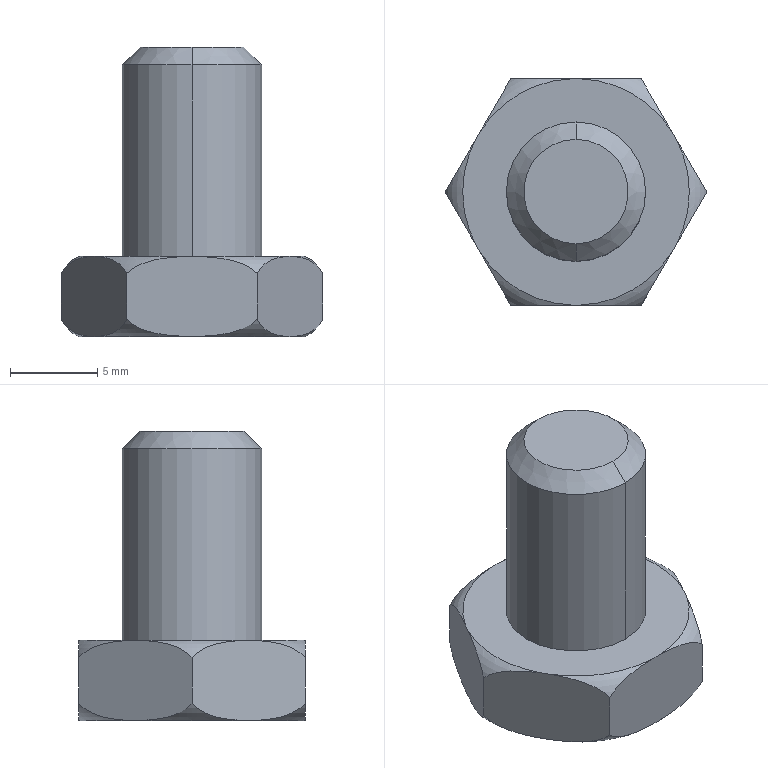Part | NX | features solid 2 | 1 solid | 25 faces | box 15.011 x 13 x 16.6 mm | volume 1260 mm3 | torus 12 | plane 9 | cylinder 2 | cone 2 | commonest cylinder face diameters 8 x2
STEP:
#1=CARTESIAN_POINT('',(280.505,2120.638,-1073.6));
#2=VERTEX_POINT('',#1);
#3=CARTESIAN_POINT('',(280.236,2120.172,-1073.6));
#4=VERTEX_POINT('',#3);
#5=CARTESIAN_POINT('',(280.505,2120.638,-1073.6));
#6=DIRECTION('',(-0.5,-0.866,0.));
#7=VECTOR('',#6,1000.);
#8=LINE('',#5,#7);
#9=EDGE_CURVE('',#2,#4,#8,.T.);
#10=ORIENTED_EDGE('',*,*,#9,.F.);
#11=CARTESIAN_POINT('',(285.731,2123.655,-1073.6));
#12=VERTEX_POINT('',#11);
#13=CARTESIAN_POINT('',(286.,2117.155,-1073.6));
#14=DIRECTION('',(0.,0.,1.));
#15=DIRECTION('',(-0.04131,0.9991,0.));
#16=AXIS2_PLACEMENT_3D('',#13,#14,#15);
#17=CIRCLE('',#16,6.506);
#18=EDGE_CURVE('',#12,#2,#17,.T.);
#19=ORIENTED_EDGE('',*,*,#18,.F.);
#20=CARTESIAN_POINT('',(286.269,2123.655,-1073.6));
#21=VERTEX_POINT('',#20);
#22=CARTESIAN_POINT('',(286.269,2123.655,-1073.6));
#23=DIRECTION('',(-1.,0.,0.));
#24=VECTOR('',#23,1000.);
#25=LINE('',#22,#24);
#26=EDGE_CURVE('',#21,#12,#25,.T.);
#27=ORIENTED_EDGE('',*,*,#26,.F.);
#28=CARTESIAN_POINT('',(291.495,2120.638,-1073.6));
#29=VERTEX_POINT('',#28);
#30=CARTESIAN_POINT('',(286.,2117.155,-1073.6));
#31=DIRECTION('',(0.,0.,1.));
#32=DIRECTION('',(0.8446,0.5353,0.));
#33=AXIS2_PLACEMENT_3D('',#30,#31,#32);
#34=CIRCLE('',#33,6.506);
#35=EDGE_CURVE('',#29,#21,#34,.T.);
#36=ORIENTED_EDGE('',*,*,#35,.F.);
#37=CARTESIAN_POINT('',(291.764,2120.172,-1073.6));
#38=VERTEX_POINT('',#37);
#39=CARTESIAN_POINT('',(291.764,2120.172,-1073.6));
#40=DIRECTION('',(-0.5,0.866,0.));
#41=VECTOR('',#40,1000.);
#42=LINE('',#39,#41);
#43=EDGE_CURVE('',#38,#29,#42,.T.);
#44=ORIENTED_EDGE('',*,*,#43,.F.);
#45=CARTESIAN_POINT('',(292.506,2117.155,-1073.6));
#46=VERTEX_POINT('',#45);
#47=CARTESIAN_POINT('',(286.,2117.155,-1073.6));
#48=DIRECTION('',(0.,0.,1.));
#49=DIRECTION('',(1.,0.,0.));
#50=AXIS2_PLACEMENT_3D('',#47,#48,#49);
#51=CIRCLE('',#50,6.506);
#52=EDGE_CURVE('',#46,#38,#51,.T.);
#53=ORIENTED_EDGE('',*,*,#52,.F.);
#54=CARTESIAN_POINT('',(291.764,2114.138,-1073.6));
#55=VERTEX_POINT('',#54);
#56=CARTESIAN_POINT('',(286.,2117.155,-1073.6));
#57=DIRECTION('',(0.,0.,1.));
#58=DIRECTION('',(0.8859,-0.4638,0.));
#59=AXIS2_PLACEMENT_3D('',#56,#57,#58);
#60=CIRCLE('',#59,6.506);
#61=EDGE_CURVE('',#55,#46,#60,.T.);
#62=ORIENTED_EDGE('',*,*,#61,.F.);
#63=CARTESIAN_POINT('',(291.495,2113.672,-1073.6));
#64=VERTEX_POINT('',#63);
#65=CARTESIAN_POINT('',(291.495,2113.672,-1073.6));
#66=DIRECTION('',(0.5,0.866,0.));
#67=VECTOR('',#66,1000.);
#68=LINE('',#65,#67);
#69=EDGE_CURVE('',#64,#55,#68,.T.);
#70=ORIENTED_EDGE('',*,*,#69,.F.);
#71=CARTESIAN_POINT('',(286.269,2110.655,-1073.6));
#72=VERTEX_POINT('',#71);
#73=CARTESIAN_POINT('',(286.,2117.155,-1073.6));
#74=DIRECTION('',(0.,0.,1.));
#75=DIRECTION('',(0.04131,-0.9991,0.));
#76=AXIS2_PLACEMENT_3D('',#73,#74,#75);
#77=CIRCLE('',#76,6.506);
#78=EDGE_CURVE('',#72,#64,#77,.T.);
#79=ORIENTED_EDGE('',*,*,#78,.F.);
#80=CARTESIAN_POINT('',(285.731,2110.655,-1073.6));
#81=VERTEX_POINT('',#80);
#82=CARTESIAN_POINT('',(285.731,2110.655,-1073.6));
#83=DIRECTION('',(1.,0.,0.));
#84=VECTOR('',#83,1000.);
#85=LINE('',#82,#84);
#86=EDGE_CURVE('',#81,#72,#85,.T.);
#87=ORIENTED_EDGE('',*,*,#86,.F.);
#88=CARTESIAN_POINT('',(280.505,2113.672,-1073.6));
#89=VERTEX_POINT('',#88);
#90=CARTESIAN_POINT('',(286.,2117.155,-1073.6));
#91=DIRECTION('',(0.,0.,1.));
#92=DIRECTION('',(-0.8446,-0.5353,0.));
#93=AXIS2_PLACEMENT_3D('',#90,#91,#92);
#94=CIRCLE('',#93,6.506);
#95=EDGE_CURVE('',#89,#81,#94,.T.);
#96=ORIENTED_EDGE('',*,*,#95,.F.);
#97=CARTESIAN_POINT('',(280.236,2114.138,-1073.6));
#98=VERTEX_POINT('',#97);
#99=CARTESIAN_POINT('',(280.236,2114.138,-1073.6));
#100=DIRECTION('',(0.5,-0.866,0.));
#101=VECTOR('',#100,1000.);
#102=LINE('',#99,#101);
#103=EDGE_CURVE('',#98,#89,#102,.T.);
#104=ORIENTED_EDGE('',*,*,#103,.F.);
#105=CARTESIAN_POINT('',(279.494,2117.155,-1073.6));
#106=VERTEX_POINT('',#105);
#107=CARTESIAN_POINT('',(286.,2117.155,-1073.6));
#108=DIRECTION('',(0.,0.,1.));
#109=DIRECTION('',(-1.,0.,0.));
#110=AXIS2_PLACEMENT_3D('',#107,#108,#109);
#111=CIRCLE('',#110,6.506);
#112=EDGE_CURVE('',#106,#98,#111,.T.);
#113=ORIENTED_EDGE('',*,*,#112,.F.);
#114=CARTESIAN_POINT('',(286.,2117.155,-1073.6));
#115=DIRECTION('',(0.,0.,1.));
#116=DIRECTION('',(-0.8859,0.4638,0.));
#117=AXIS2_PLACEMENT_3D('',#114,#115,#116);
#118=CIRCLE('',#117,6.506);
#119=EDGE_CURVE('',#4,#106,#118,.T.);
#120=ORIENTED_EDGE('',*,*,#119,.F.);
#121=EDGE_LOOP('',(#10,#19,#27,#36,#44,#53,#62,#70,#79,#87,#96,#104,#113,#120));
#122=FACE_BOUND('',#121,.T.);
#123=CARTESIAN_POINT('',(286.,2117.155,-1073.6));
#124=DIRECTION('',(0.,0.,1.));
#125=DIRECTION('',(1.,0.,0.));
#126=AXIS2_PLACEMENT_3D('',#123,#124,#125);
#127=PLANE('',#126);
#128=ADVANCED_FACE('',(#122),#127,.F.);
#129=CARTESIAN_POINT('',(278.494,2117.155,-1072.6));
#130=VERTEX_POINT('',#129);
#131=CARTESIAN_POINT('',(278.494,2117.155,-1072.6));
#132=CARTESIAN_POINT('',(278.513,2117.123,-1072.641));
#133=CARTESIAN_POINT('',(278.553,2117.053,-1072.722));
#134=CARTESIAN_POINT('',(278.626,2116.927,-1072.843));
#135=CARTESIAN_POINT('',(278.713,2116.776,-1072.962));
#136=CARTESIAN_POINT('',(278.817,2116.596,-1073.079));
#137=CARTESIAN_POINT('',(278.94,2116.383,-1073.191));
#138=CARTESIAN_POINT('',(279.081,2116.139,-1073.292));
#139=CARTESIAN_POINT('',(279.239,2115.866,-1073.381));
#140=CARTESIAN_POINT('',(279.413,2115.565,-1073.455));
#141=CARTESIAN_POINT('',(279.602,2115.236,-1073.514));
#142=CARTESIAN_POINT('',(279.805,2114.886,-1073.558));
#143=CARTESIAN_POINT('',(280.017,2114.517,-1073.587));
#144=CARTESIAN_POINT('',(280.163,2114.266,-1073.597));
#145=CARTESIAN_POINT('',(280.236,2114.138,-1073.6));
#146=B_SPLINE_CURVE_WITH_KNOTS('',3,(#131,#132,#133,#134,#135,#136,#137,#138,#139,#140,#141,#142,#143,#144,#145),.UNSPECIFIED.,.F.,.F.,(4,1,1,1,1,1,1,1,1,1,1,1,4),(0.,0.08333,0.1667,0.25,0.3333,0.4167,0.5,0.5833,0.6667,0.75,0.8333,0.9167,1.),.QUASI_UNIFORM_KNOTS.);
#147=EDGE_CURVE('',#130,#98,#146,.T.);
#148=ORIENTED_EDGE('',*,*,#147,.F.);
#149=CARTESIAN_POINT('',(278.494,2117.155,-1072.6));
#150=CARTESIAN_POINT('',(278.513,2117.187,-1072.641));
#151=CARTESIAN_POINT('',(278.553,2117.257,-1072.722));
#152=CARTESIAN_POINT('',(278.626,2117.383,-1072.843));
#153=CARTESIAN_POINT('',(278.713,2117.534,-1072.962));
#154=CARTESIAN_POINT('',(278.817,2117.715,-1073.079));
#155=CARTESIAN_POINT('',(278.94,2117.927,-1073.191));
#156=CARTESIAN_POINT('',(279.081,2118.171,-1073.292));
#157=CARTESIAN_POINT('',(279.239,2118.444,-1073.381));
#158=CARTESIAN_POINT('',(279.413,2118.745,-1073.455));
#159=CARTESIAN_POINT('',(279.602,2119.074,-1073.514));
#160=CARTESIAN_POINT('',(279.805,2119.424,-1073.558));
#161=CARTESIAN_POINT('',(280.017,2119.793,-1073.587));
#162=CARTESIAN_POINT('',(280.163,2120.044,-1073.597));
#163=CARTESIAN_POINT('',(280.236,2120.172,-1073.6));
#164=B_SPLINE_CURVE_WITH_KNOTS('',3,(#149,#150,#151,#152,#153,#154,#155,#156,#157,#158,#159,#160,#161,#162,#163),.UNSPECIFIED.,.F.,.F.,(4,1,1,1,1,1,1,1,1,1,1,1,4),(0.,0.08333,0.1667,0.25,0.3333,0.4167,0.5,0.5833,0.6667,0.75,0.8333,0.9167,1.),.QUASI_UNIFORM_KNOTS.);
#165=EDGE_CURVE('',#130,#4,#164,.T.);
#166=ORIENTED_EDGE('',*,*,#165,.T.);
#167=ORIENTED_EDGE('',*,*,#119,.T.);
#168=ORIENTED_EDGE('',*,*,#112,.T.);
#169=EDGE_LOOP('',(#148,#166,#167,#168));
#170=FACE_BOUND('',#169,.T.);
#171=CARTESIAN_POINT('',(286.,2117.155,-1071.777));
#172=DIRECTION('',(0.,0.,1.));
#173=DIRECTION('',(1.,0.,0.));
#174=AXIS2_PLACEMENT_3D('',#171,#172,#173);
#175=TOROIDAL_SURFACE('',#174,5.683,2.);
#176=ADVANCED_FACE('',(#170),#175,.T.);
#177=CARTESIAN_POINT('',(280.236,2120.172,-1069.));
#178=VERTEX_POINT('',#177);
#179=CARTESIAN_POINT('',(280.505,2120.638,-1069.));
#180=VERTEX_POINT('',#179);
#181=CARTESIAN_POINT('',(280.236,2120.172,-1069.));
#182=DIRECTION('',(0.5,0.866,0.));
#183=VECTOR('',#182,1000.);
#184=LINE('',#181,#183);
#185=EDGE_CURVE('',#178,#180,#184,.T.);
#186=ORIENTED_EDGE('',*,*,#185,.T.);
#187=CARTESIAN_POINT('',(282.247,2123.655,-1070.));
#188=VERTEX_POINT('',#187);
#189=CARTESIAN_POINT('',(282.247,2123.655,-1070.));
#190=CARTESIAN_POINT('',(282.229,2123.623,-1069.959));
#191=CARTESIAN_POINT('',(282.188,2123.553,-1069.878));
#192=CARTESIAN_POINT('',(282.116,2123.427,-1069.757));
#193=CARTESIAN_POINT('',(282.028,2123.276,-1069.638));
#194=CARTESIAN_POINT('',(281.924,2123.095,-1069.521));
#195=CARTESIAN_POINT('',(281.801,2122.883,-1069.409));
#196=CARTESIAN_POINT('',(281.66,2122.639,-1069.308));
#197=CARTESIAN_POINT('',(281.503,2122.366,-1069.219));
#198=CARTESIAN_POINT('',(281.329,2122.065,-1069.145));
#199=CARTESIAN_POINT('',(281.139,2121.736,-1069.086));
#200=CARTESIAN_POINT('',(280.937,2121.386,-1069.042));
#201=CARTESIAN_POINT('',(280.724,2121.017,-1069.013));
#202=CARTESIAN_POINT('',(280.579,2120.766,-1069.003));
#203=CARTESIAN_POINT('',(280.505,2120.638,-1069.));
#204=B_SPLINE_CURVE_WITH_KNOTS('',3,(#189,#190,#191,#192,#193,#194,#195,#196,#197,#198,#199,#200,#201,#202,#203),.UNSPECIFIED.,.F.,.F.,(4,1,1,1,1,1,1,1,1,1,1,1,4),(0.,0.08333,0.1667,0.25,0.3333,0.4167,0.5,0.5833,0.6667,0.75,0.8333,0.9167,1.),.QUASI_UNIFORM_KNOTS.);
#205=EDGE_CURVE('',#188,#180,#204,.T.);
#206=ORIENTED_EDGE('',*,*,#205,.F.);
#207=CARTESIAN_POINT('',(282.247,2123.655,-1072.6));
#208=VERTEX_POINT('',#207);
#209=CARTESIAN_POINT('',(282.247,2123.655,-1072.6));
#210=DIRECTION('',(0.,0.,1.));
#211=VECTOR('',#210,1000.);
#212=LINE('',#209,#211);
#213=EDGE_CURVE('',#208,#188,#212,.T.);
#214=ORIENTED_EDGE('',*,*,#213,.F.);
#215=CARTESIAN_POINT('',(282.247,2123.655,-1072.6));
#216=CARTESIAN_POINT('',(282.229,2123.623,-1072.641));
#217=CARTESIAN_POINT('',(282.188,2123.553,-1072.722));
#218=CARTESIAN_POINT('',(282.116,2123.427,-1072.843));
#219=CARTESIAN_POINT('',(282.028,2123.276,-1072.962));
#220=CARTESIAN_POINT('',(281.924,2123.096,-1073.079));
#221=CARTESIAN_POINT('',(281.801,2122.883,-1073.191));
#222=CARTESIAN_POINT('',(281.66,2122.639,-1073.292));
#223=CARTESIAN_POINT('',(281.503,2122.366,-1073.381));
#224=CARTESIAN_POINT('',(281.329,2122.065,-1073.455));
#225=CARTESIAN_POINT('',(281.139,2121.736,-1073.514));
#226=CARTESIAN_POINT('',(280.937,2121.386,-1073.558));
#227=CARTESIAN_POINT('',(280.724,2121.017,-1073.587));
#228=CARTESIAN_POINT('',(280.579,2120.766,-1073.597));
#229=CARTESIAN_POINT('',(280.505,2120.638,-1073.6));
#230=B_SPLINE_CURVE_WITH_KNOTS('',3,(#215,#216,#217,#218,#219,#220,#221,#222,#223,#224,#225,#226,#227,#228,#229),.UNSPECIFIED.,.F.,.F.,(4,1,1,1,1,1,1,1,1,1,1,1,4),(0.,0.08333,0.1667,0.25,0.3333,0.4167,0.5,0.5833,0.6667,0.75,0.8333,0.9167,1.),.QUASI_UNIFORM_KNOTS.);
#231=EDGE_CURVE('',#208,#2,#230,.T.);
#232=ORIENTED_EDGE('',*,*,#231,.T.);
#233=ORIENTED_EDGE('',*,*,#9,.T.);
#234=ORIENTED_EDGE('',*,*,#165,.F.);
#235=CARTESIAN_POINT('',(278.494,2117.155,-1070.));
#236=VERTEX_POINT('',#235);
#237=CARTESIAN_POINT('',(278.494,2117.155,-1072.6));
#238=DIRECTION('',(0.,0.,1.));
#239=VECTOR('',#238,1000.);
#240=LINE('',#237,#239);
#241=EDGE_CURVE('',#130,#236,#240,.T.);
#242=ORIENTED_EDGE('',*,*,#241,.T.);
#243=CARTESIAN_POINT('',(278.494,2117.155,-1070.));
#244=CARTESIAN_POINT('',(278.513,2117.187,-1069.959));
#245=CARTESIAN_POINT('',(278.553,2117.257,-1069.878));
#246=CARTESIAN_POINT('',(278.626,2117.383,-1069.757));
#247=CARTESIAN_POINT('',(278.713,2117.534,-1069.638));
#248=CARTESIAN_POINT('',(278.817,2117.714,-1069.521));
#249=CARTESIAN_POINT('',(278.94,2117.927,-1069.409));
#250=CARTESIAN_POINT('',(279.081,2118.171,-1069.308));
#251=CARTESIAN_POINT('',(279.239,2118.444,-1069.219));
#252=CARTESIAN_POINT('',(279.413,2118.745,-1069.145));
#253=CARTESIAN_POINT('',(279.602,2119.074,-1069.086));
#254=CARTESIAN_POINT('',(279.805,2119.424,-1069.042));
#255=CARTESIAN_POINT('',(280.017,2119.793,-1069.013));
#256=CARTESIAN_POINT('',(280.163,2120.044,-1069.003));
#257=CARTESIAN_POINT('',(280.236,2120.172,-1069.));
#258=B_SPLINE_CURVE_WITH_KNOTS('',3,(#243,#244,#245,#246,#247,#248,#249,#250,#251,#252,#253,#254,#255,#256,#257),.UNSPECIFIED.,.F.,.F.,(4,1,1,1,1,1,1,1,1,1,1,1,4),(0.,0.08333,0.1667,0.25,0.3333,0.4167,0.5,0.5833,0.6667,0.75,0.8333,0.9167,1.),.QUASI_UNIFORM_KNOTS.);
#259=EDGE_CURVE('',#236,#178,#258,.T.);
#260=ORIENTED_EDGE('',*,*,#259,.T.);
#261=EDGE_LOOP('',(#186,#206,#214,#232,#233,#234,#242,#260));
#262=FACE_BOUND('',#261,.T.);
#263=CARTESIAN_POINT('',(282.247,2123.655,-1073.6));
#264=DIRECTION('',(-0.866,0.5,0.));
#265=DIRECTION('',(0.5,0.866,0.));
#266=AXIS2_PLACEMENT_3D('',#263,#264,#265);
#267=PLANE('',#266);
#268=ADVANCED_FACE('',(#262),#267,.T.);
#269=CARTESIAN_POINT('',(280.236,2114.138,-1069.));
#270=VERTEX_POINT('',#269);
#271=CARTESIAN_POINT('',(279.494,2117.155,-1069.));
#272=VERTEX_POINT('',#271);
#273=CARTESIAN_POINT('',(286.,2117.155,-1069.));
#274=DIRECTION('',(0.,0.,-1.));
#275=DIRECTION('',(-0.8859,-0.4638,0.));
#276=AXIS2_PLACEMENT_3D('',#273,#274,#275);
#277=CIRCLE('',#276,6.506);
#278=EDGE_CURVE('',#270,#272,#277,.T.);
#279=ORIENTED_EDGE('',*,*,#278,.T.);
#280=CARTESIAN_POINT('',(286.,2117.155,-1069.));
#281=DIRECTION('',(0.,0.,-1.));
#282=DIRECTION('',(-1.,0.,0.));
#283=AXIS2_PLACEMENT_3D('',#280,#281,#282);
#284=CIRCLE('',#283,6.506);
#285=EDGE_CURVE('',#272,#178,#284,.T.);
#286=ORIENTED_EDGE('',*,*,#285,.T.);
#287=ORIENTED_EDGE('',*,*,#259,.F.);
#288=CARTESIAN_POINT('',(278.494,2117.155,-1070.));
#289=CARTESIAN_POINT('',(278.513,2117.123,-1069.959));
#290=CARTESIAN_POINT('',(278.553,2117.053,-1069.878));
#291=CARTESIAN_POINT('',(278.626,2116.927,-1069.757));
#292=CARTESIAN_POINT('',(278.713,2116.776,-1069.638));
#293=CARTESIAN_POINT('',(278.817,2116.595,-1069.521));
#294=CARTESIAN_POINT('',(278.94,2116.383,-1069.409));
#295=CARTESIAN_POINT('',(279.081,2116.139,-1069.308));
#296=CARTESIAN_POINT('',(279.239,2115.866,-1069.219));
#297=CARTESIAN_POINT('',(279.413,2115.565,-1069.145));
#298=CARTESIAN_POINT('',(279.602,2115.236,-1069.086));
#299=CARTESIAN_POINT('',(279.805,2114.886,-1069.042));
#300=CARTESIAN_POINT('',(280.017,2114.517,-1069.013));
#301=CARTESIAN_POINT('',(280.163,2114.266,-1069.003));
#302=CARTESIAN_POINT('',(280.236,2114.138,-1069.));
#303=B_SPLINE_CURVE_WITH_KNOTS('',3,(#288,#289,#290,#291,#292,#293,#294,#295,#296,#297,#298,#299,#300,#301,#302),.UNSPECIFIED.,.F.,.F.,(4,1,1,1,1,1,1,1,1,1,1,1,4),(0.,0.08333,0.1667,0.25,0.3333,0.4167,0.5,0.5833,0.6667,0.75,0.8333,0.9167,1.),.QUASI_UNIFORM_KNOTS.);
#304=EDGE_CURVE('',#236,#270,#303,.T.);
#305=ORIENTED_EDGE('',*,*,#304,.T.);
#306=EDGE_LOOP('',(#279,#286,#287,#305));
#307=FACE_BOUND('',#306,.T.);
#308=CARTESIAN_POINT('',(286.,2117.155,-1070.823));
#309=DIRECTION('',(0.,0.,1.));
#310=DIRECTION('',(1.,0.,0.));
#311=AXIS2_PLACEMENT_3D('',#308,#309,#310);
#312=TOROIDAL_SURFACE('',#311,5.683,2.);
#313=ADVANCED_FACE('',(#307),#312,.T.);
#314=CARTESIAN_POINT('',(280.505,2113.672,-1069.));
#315=VERTEX_POINT('',#314);
#316=CARTESIAN_POINT('',(280.505,2113.672,-1069.));
#317=DIRECTION('',(-0.5,0.866,0.));
#318=VECTOR('',#317,1000.);
#319=LINE('',#316,#318);
#320=EDGE_CURVE('',#315,#270,#319,.T.);
#321=ORIENTED_EDGE('',*,*,#320,.T.);
#322=ORIENTED_EDGE('',*,*,#304,.F.);
#323=ORIENTED_EDGE('',*,*,#241,.F.);
#324=ORIENTED_EDGE('',*,*,#147,.T.);
#325=ORIENTED_EDGE('',*,*,#103,.T.);
#326=CARTESIAN_POINT('',(282.247,2110.655,-1072.6));
#327=VERTEX_POINT('',#326);
#328=CARTESIAN_POINT('',(282.247,2110.655,-1072.6));
#329=CARTESIAN_POINT('',(282.229,2110.687,-1072.641));
#330=CARTESIAN_POINT('',(282.188,2110.757,-1072.722));
#331=CARTESIAN_POINT('',(282.116,2110.883,-1072.843));
#332=CARTESIAN_POINT('',(282.028,2111.034,-1072.962));
#333=CARTESIAN_POINT('',(281.924,2111.215,-1073.079));
#334=CARTESIAN_POINT('',(281.801,2111.427,-1073.191));
#335=CARTESIAN_POINT('',(281.66,2111.671,-1073.292));
#336=CARTESIAN_POINT('',(281.503,2111.944,-1073.381));
#337=CARTESIAN_POINT('',(281.329,2112.245,-1073.455));
#338=CARTESIAN_POINT('',(281.139,2112.574,-1073.514));
#339=CARTESIAN_POINT('',(280.937,2112.924,-1073.558));
#340=CARTESIAN_POINT('',(280.724,2113.293,-1073.587));
#341=CARTESIAN_POINT('',(280.579,2113.544,-1073.597));
#342=CARTESIAN_POINT('',(280.505,2113.672,-1073.6));
#343=B_SPLINE_CURVE_WITH_KNOTS('',3,(#328,#329,#330,#331,#332,#333,#334,#335,#336,#337,#338,#339,#340,#341,#342),.UNSPECIFIED.,.F.,.F.,(4,1,1,1,1,1,1,1,1,1,1,1,4),(0.,0.08333,0.1667,0.25,0.3333,0.4167,0.5,0.5833,0.6667,0.75,0.8333,0.9167,1.),.QUASI_UNIFORM_KNOTS.);
#344=EDGE_CURVE('',#327,#89,#343,.T.);
#345=ORIENTED_EDGE('',*,*,#344,.F.);
#346=CARTESIAN_POINT('',(282.247,2110.655,-1070.));
#347=VERTEX_POINT('',#346);
#348=CARTESIAN_POINT('',(282.247,2110.655,-1072.6));
#349=DIRECTION('',(0.,0.,1.));
#350=VECTOR('',#349,1000.);
#351=LINE('',#348,#350);
#352=EDGE_CURVE('',#327,#347,#351,.T.);
#353=ORIENTED_EDGE('',*,*,#352,.T.);
#354=CARTESIAN_POINT('',(282.247,2110.655,-1070.));
#355=CARTESIAN_POINT('',(282.229,2110.687,-1069.959));
#356=CARTESIAN_POINT('',(282.188,2110.757,-1069.878));
#357=CARTESIAN_POINT('',(282.116,2110.883,-1069.757));
#358=CARTESIAN_POINT('',(282.028,2111.034,-1069.638));
#359=CARTESIAN_POINT('',(281.924,2111.214,-1069.521));
#360=CARTESIAN_POINT('',(281.801,2111.427,-1069.409));
#361=CARTESIAN_POINT('',(281.66,2111.671,-1069.308));
#362=CARTESIAN_POINT('',(281.503,2111.944,-1069.219));
#363=CARTESIAN_POINT('',(281.329,2112.245,-1069.145));
#364=CARTESIAN_POINT('',(281.139,2112.574,-1069.086));
#365=CARTESIAN_POINT('',(280.937,2112.924,-1069.042));
#366=CARTESIAN_POINT('',(280.724,2113.293,-1069.013));
#367=CARTESIAN_POINT('',(280.579,2113.544,-1069.003));
#368=CARTESIAN_POINT('',(280.505,2113.672,-1069.));
#369=B_SPLINE_CURVE_WITH_KNOTS('',3,(#354,#355,#356,#357,#358,#359,#360,#361,#362,#363,#364,#365,#366,#367,#368),.UNSPECIFIED.,.F.,.F.,(4,1,1,1,1,1,1,1,1,1,1,1,4),(0.,0.08333,0.1667,0.25,0.3333,0.4167,0.5,0.5833,0.6667,0.75,0.8333,0.9167,1.),.QUASI_UNIFORM_KNOTS.);
#370=EDGE_CURVE('',#347,#315,#369,.T.);
#371=ORIENTED_EDGE('',*,*,#370,.T.);
#372=EDGE_LOOP('',(#321,#322,#323,#324,#325,#345,#353,#371));
#373=FACE_BOUND('',#372,.T.);
#374=CARTESIAN_POINT('',(278.494,2117.155,-1073.6));
#375=DIRECTION('',(-0.866,-0.5,0.));
#376=DIRECTION('',(-0.5,0.866,0.));
#377=AXIS2_PLACEMENT_3D('',#374,#375,#376);
#378=PLANE('',#377);
#379=ADVANCED_FACE('',(#373),#378,.T.);
#380=ORIENTED_EDGE('',*,*,#370,.F.);
#381=CARTESIAN_POINT('',(285.731,2110.655,-1069.));
#382=VERTEX_POINT('',#381);
#383=CARTESIAN_POINT('',(282.247,2110.655,-1070.));
#384=CARTESIAN_POINT('',(282.284,2110.655,-1069.959));
#385=CARTESIAN_POINT('',(282.365,2110.655,-1069.878));
#386=CARTESIAN_POINT('',(282.51,2110.655,-1069.757));
#387=CARTESIAN_POINT('',(282.685,2110.655,-1069.638));
#388=CARTESIAN_POINT('',(282.893,2110.655,-1069.521));
#389=CARTESIAN_POINT('',(283.139,2110.655,-1069.409));
#390=CARTESIAN_POINT('',(283.421,2110.655,-1069.308));
#391=CARTESIAN_POINT('',(283.736,2110.655,-1069.219));
#392=CARTESIAN_POINT('',(284.084,2110.655,-1069.145));
#393=CARTESIAN_POINT('',(284.463,2110.655,-1069.086));
#394=CARTESIAN_POINT('',(284.868,2110.655,-1069.042));
#395=CARTESIAN_POINT('',(285.293,2110.655,-1069.013));
#396=CARTESIAN_POINT('',(285.584,2110.655,-1069.003));
#397=CARTESIAN_POINT('',(285.731,2110.655,-1069.));
#398=B_SPLINE_CURVE_WITH_KNOTS('',3,(#383,#384,#385,#386,#387,#388,#389,#390,#391,#392,#393,#394,#395,#396,#397),.UNSPECIFIED.,.F.,.F.,(4,1,1,1,1,1,1,1,1,1,1,1,4),(0.,0.08333,0.1667,0.25,0.3333,0.4167,0.5,0.5833,0.6667,0.75,0.8333,0.9167,1.),.QUASI_UNIFORM_KNOTS.);
#399=EDGE_CURVE('',#347,#382,#398,.T.);
#400=ORIENTED_EDGE('',*,*,#399,.T.);
#401=CARTESIAN_POINT('',(286.,2117.155,-1069.));
#402=DIRECTION('',(0.,0.,-1.));
#403=DIRECTION('',(-0.04131,-0.9991,0.));
#404=AXIS2_PLACEMENT_3D('',#401,#402,#403);
#405=CIRCLE('',#404,6.506);
#406=EDGE_CURVE('',#382,#315,#405,.T.);
#407=ORIENTED_EDGE('',*,*,#406,.T.);
#408=EDGE_LOOP('',(#380,#400,#407));
#409=FACE_BOUND('',#408,.T.);
#410=CARTESIAN_POINT('',(286.,2117.155,-1070.823));
#411=DIRECTION('',(0.,0.,1.));
#412=DIRECTION('',(1.,0.,0.));
#413=AXIS2_PLACEMENT_3D('',#410,#411,#412);
#414=TOROIDAL_SURFACE('',#413,5.683,2.);
#415=ADVANCED_FACE('',(#409),#414,.T.);
#416=ORIENTED_EDGE('',*,*,#320,.F.);
#417=ORIENTED_EDGE('',*,*,#406,.F.);
#418=CARTESIAN_POINT('',(286.269,2110.655,-1069.));
#419=VERTEX_POINT('',#418);
#420=CARTESIAN_POINT('',(285.731,2110.655,-1069.));
#421=DIRECTION('',(1.,0.,0.));
#422=VECTOR('',#421,1000.);
#423=LINE('',#420,#422);
#424=EDGE_CURVE('',#382,#419,#423,.T.);
#425=ORIENTED_EDGE('',*,*,#424,.T.);
#426=CARTESIAN_POINT('',(291.495,2113.672,-1069.));
#427=VERTEX_POINT('',#426);
#428=CARTESIAN_POINT('',(286.,2117.155,-1069.));
#429=DIRECTION('',(0.,0.,-1.));
#430=DIRECTION('',(0.8446,-0.5353,0.));
#431=AXIS2_PLACEMENT_3D('',#428,#429,#430);
#432=CIRCLE('',#431,6.506);
#433=EDGE_CURVE('',#427,#419,#432,.T.);
#434=ORIENTED_EDGE('',*,*,#433,.F.);
#435=CARTESIAN_POINT('',(291.764,2114.138,-1069.));
#436=VERTEX_POINT('',#435);
#437=CARTESIAN_POINT('',(291.764,2114.138,-1069.));
#438=DIRECTION('',(-0.5,-0.866,0.));
#439=VECTOR('',#438,1000.);
#440=LINE('',#437,#439);
#441=EDGE_CURVE('',#436,#427,#440,.T.);
#442=ORIENTED_EDGE('',*,*,#441,.F.);
#443=CARTESIAN_POINT('',(292.506,2117.155,-1069.));
#444=VERTEX_POINT('',#443);
#445=CARTESIAN_POINT('',(286.,2117.155,-1069.));
#446=DIRECTION('',(0.,0.,-1.));
#447=DIRECTION('',(1.,0.,0.));
#448=AXIS2_PLACEMENT_3D('',#445,#446,#447);
#449=CIRCLE('',#448,6.506);
#450=EDGE_CURVE('',#444,#436,#449,.T.);
#451=ORIENTED_EDGE('',*,*,#450,.F.);
#452=CARTESIAN_POINT('',(291.764,2120.172,-1069.));
#453=VERTEX_POINT('',#452);
#454=CARTESIAN_POINT('',(286.,2117.155,-1069.));
#455=DIRECTION('',(0.,0.,-1.));
#456=DIRECTION('',(0.8859,0.4638,0.));
#457=AXIS2_PLACEMENT_3D('',#454,#455,#456);
#458=CIRCLE('',#457,6.506);
#459=EDGE_CURVE('',#453,#444,#458,.T.);
#460=ORIENTED_EDGE('',*,*,#459,.F.);
#461=CARTESIAN_POINT('',(291.495,2120.638,-1069.));
#462=VERTEX_POINT('',#461);
#463=CARTESIAN_POINT('',(291.495,2120.638,-1069.));
#464=DIRECTION('',(0.5,-0.866,0.));
#465=VECTOR('',#464,1000.);
#466=LINE('',#463,#465);
#467=EDGE_CURVE('',#462,#453,#466,.T.);
#468=ORIENTED_EDGE('',*,*,#467,.F.);
#469=CARTESIAN_POINT('',(286.269,2123.655,-1069.));
#470=VERTEX_POINT('',#469);
#471=CARTESIAN_POINT('',(286.,2117.155,-1069.));
#472=DIRECTION('',(0.,0.,-1.));
#473=DIRECTION('',(0.04131,0.9991,0.));
#474=AXIS2_PLACEMENT_3D('',#471,#472,#473);
#475=CIRCLE('',#474,6.506);
#476=EDGE_CURVE('',#470,#462,#475,.T.);
#477=ORIENTED_EDGE('',*,*,#476,.F.);
#478=CARTESIAN_POINT('',(285.731,2123.655,-1069.));
#479=VERTEX_POINT('',#478);
#480=CARTESIAN_POINT('',(286.269,2123.655,-1069.));
#481=DIRECTION('',(-1.,0.,0.));
#482=VECTOR('',#481,1000.);
#483=LINE('',#480,#482);
#484=EDGE_CURVE('',#470,#479,#483,.T.);
#485=ORIENTED_EDGE('',*,*,#484,.T.);
#486=CARTESIAN_POINT('',(286.,2117.155,-1069.));
#487=DIRECTION('',(0.,0.,-1.));
#488=DIRECTION('',(-0.8446,0.5353,0.));
#489=AXIS2_PLACEMENT_3D('',#486,#487,#488);
#490=CIRCLE('',#489,6.506);
#491=EDGE_CURVE('',#180,#479,#490,.T.);
#492=ORIENTED_EDGE('',*,*,#491,.F.);
#493=ORIENTED_EDGE('',*,*,#185,.F.);
#494=ORIENTED_EDGE('',*,*,#285,.F.);
#495=ORIENTED_EDGE('',*,*,#278,.F.);
#496=EDGE_LOOP('',(#416,#417,#425,#434,#442,#451,#460,#468,#477,#485,#492,#493,#494,#495));
#497=FACE_BOUND('',#496,.T.);
#498=CARTESIAN_POINT('',(286.,2121.155,-1069.));
#499=VERTEX_POINT('',#498);
#500=CARTESIAN_POINT('',(286.,2113.155,-1069.));
#501=VERTEX_POINT('',#500);
#502=CARTESIAN_POINT('',(286.,2117.155,-1069.));
#503=DIRECTION('',(0.,0.,1.));
#504=DIRECTION('',(0.,1.,0.));
#505=AXIS2_PLACEMENT_3D('',#502,#503,#504);
#506=CIRCLE('',#505,4.);
#507=EDGE_CURVE('',#499,#501,#506,.T.);
#508=ORIENTED_EDGE('',*,*,#507,.F.);
#509=CARTESIAN_POINT('',(286.,2117.155,-1069.));
#510=DIRECTION('',(0.,0.,1.));
#511=DIRECTION('',(0.,-1.,0.));
#512=AXIS2_PLACEMENT_3D('',#509,#510,#511);
#513=CIRCLE('',#512,4.);
#514=EDGE_CURVE('',#501,#499,#513,.T.);
#515=ORIENTED_EDGE('',*,*,#514,.F.);
#516=EDGE_LOOP('',(#508,#515));
#517=FACE_BOUND('',#516,.T.);
#518=CARTESIAN_POINT('',(286.,2117.155,-1069.));
#519=DIRECTION('',(0.,0.,1.));
#520=DIRECTION('',(1.,0.,0.));
#521=AXIS2_PLACEMENT_3D('',#518,#519,#520);
#522=PLANE('',#521);
#523=ADVANCED_FACE('',(#497,#517),#522,.T.);
#524=CARTESIAN_POINT('',(282.247,2123.655,-1070.));
#525=CARTESIAN_POINT('',(282.284,2123.655,-1069.959));
#526=CARTESIAN_POINT('',(282.365,2123.655,-1069.878));
#527=CARTESIAN_POINT('',(282.51,2123.655,-1069.757));
#528=CARTESIAN_POINT('',(282.685,2123.655,-1069.638));
#529=CARTESIAN_POINT('',(282.893,2123.655,-1069.521));
#530=CARTESIAN_POINT('',(283.139,2123.655,-1069.409));
#531=CARTESIAN_POINT('',(283.421,2123.655,-1069.308));
#532=CARTESIAN_POINT('',(283.736,2123.655,-1069.219));
#533=CARTESIAN_POINT('',(284.084,2123.655,-1069.145));
#534=CARTESIAN_POINT('',(284.463,2123.655,-1069.086));
#535=CARTESIAN_POINT('',(284.868,2123.655,-1069.042));
#536=CARTESIAN_POINT('',(285.293,2123.655,-1069.013));
#537=CARTESIAN_POINT('',(285.584,2123.655,-1069.003));
#538=CARTESIAN_POINT('',(285.731,2123.655,-1069.));
#539=B_SPLINE_CURVE_WITH_KNOTS('',3,(#524,#525,#526,#527,#528,#529,#530,#531,#532,#533,#534,#535,#536,#537,#538),.UNSPECIFIED.,.F.,.F.,(4,1,1,1,1,1,1,1,1,1,1,1,4),(0.,0.08333,0.1667,0.25,0.3333,0.4167,0.5,0.5833,0.6667,0.75,0.8333,0.9167,1.),.QUASI_UNIFORM_KNOTS.);
#540=EDGE_CURVE('',#188,#479,#539,.T.);
#541=ORIENTED_EDGE('',*,*,#540,.F.);
#542=ORIENTED_EDGE('',*,*,#205,.T.);
#543=ORIENTED_EDGE('',*,*,#491,.T.);
#544=EDGE_LOOP('',(#541,#542,#543));
#545=FACE_BOUND('',#544,.T.);
#546=CARTESIAN_POINT('',(286.,2117.155,-1070.823));
#547=DIRECTION('',(0.,0.,1.));
#548=DIRECTION('',(1.,0.,0.));
#549=AXIS2_PLACEMENT_3D('',#546,#547,#548);
#550=TOROIDAL_SURFACE('',#549,5.683,2.);
#551=ADVANCED_FACE('',(#545),#550,.T.);
#552=ORIENTED_EDGE('',*,*,#484,.F.);
#553=CARTESIAN_POINT('',(289.753,2123.655,-1070.));
#554=VERTEX_POINT('',#553);
#555=CARTESIAN_POINT('',(289.753,2123.655,-1070.));
#556=CARTESIAN_POINT('',(289.716,2123.655,-1069.959));
#557=CARTESIAN_POINT('',(289.635,2123.655,-1069.878));
#558=CARTESIAN_POINT('',(289.49,2123.655,-1069.757));
#559=CARTESIAN_POINT('',(289.315,2123.655,-1069.638));
#560=CARTESIAN_POINT('',(289.107,2123.655,-1069.521));
#561=CARTESIAN_POINT('',(288.861,2123.655,-1069.409));
#562=CARTESIAN_POINT('',(288.579,2123.655,-1069.308));
#563=CARTESIAN_POINT('',(288.264,2123.655,-1069.219));
#564=CARTESIAN_POINT('',(287.916,2123.655,-1069.145));
#565=CARTESIAN_POINT('',(287.537,2123.655,-1069.086));
#566=CARTESIAN_POINT('',(287.132,2123.655,-1069.042));
#567=CARTESIAN_POINT('',(286.707,2123.655,-1069.013));
#568=CARTESIAN_POINT('',(286.416,2123.655,-1069.003));
#569=CARTESIAN_POINT('',(286.269,2123.655,-1069.));
#570=B_SPLINE_CURVE_WITH_KNOTS('',3,(#555,#556,#557,#558,#559,#560,#561,#562,#563,#564,#565,#566,#567,#568,#569),.UNSPECIFIED.,.F.,.F.,(4,1,1,1,1,1,1,1,1,1,1,1,4),(0.,0.08333,0.1667,0.25,0.3333,0.4167,0.5,0.5833,0.6667,0.75,0.8333,0.9167,1.),.QUASI_UNIFORM_KNOTS.);
#571=EDGE_CURVE('',#554,#470,#570,.T.);
#572=ORIENTED_EDGE('',*,*,#571,.F.);
#573=CARTESIAN_POINT('',(289.753,2123.655,-1072.6));
#574=VERTEX_POINT('',#573);
#575=CARTESIAN_POINT('',(289.753,2123.655,-1072.6));
#576=DIRECTION('',(0.,0.,1.));
#577=VECTOR('',#576,1000.);
#578=LINE('',#575,#577);
#579=EDGE_CURVE('',#574,#554,#578,.T.);
#580=ORIENTED_EDGE('',*,*,#579,.F.);
#581=CARTESIAN_POINT('',(289.753,2123.655,-1072.6));
#582=CARTESIAN_POINT('',(289.716,2123.655,-1072.641));
#583=CARTESIAN_POINT('',(289.635,2123.655,-1072.722));
#584=CARTESIAN_POINT('',(289.49,2123.655,-1072.843));
#585=CARTESIAN_POINT('',(289.315,2123.655,-1072.962));
#586=CARTESIAN_POINT('',(289.107,2123.655,-1073.079));
#587=CARTESIAN_POINT('',(288.861,2123.655,-1073.191));
#588=CARTESIAN_POINT('',(288.579,2123.655,-1073.292));
#589=CARTESIAN_POINT('',(288.264,2123.655,-1073.381));
#590=CARTESIAN_POINT('',(287.916,2123.655,-1073.455));
#591=CARTESIAN_POINT('',(287.537,2123.655,-1073.514));
#592=CARTESIAN_POINT('',(287.132,2123.655,-1073.558));
#593=CARTESIAN_POINT('',(286.707,2123.655,-1073.587));
#594=CARTESIAN_POINT('',(286.416,2123.655,-1073.597));
#595=CARTESIAN_POINT('',(286.269,2123.655,-1073.6));
#596=B_SPLINE_CURVE_WITH_KNOTS('',3,(#581,#582,#583,#584,#585,#586,#587,#588,#589,#590,#591,#592,#593,#594,#595),.UNSPECIFIED.,.F.,.F.,(4,1,1,1,1,1,1,1,1,1,1,1,4),(0.,0.08333,0.1667,0.25,0.3333,0.4167,0.5,0.5833,0.6667,0.75,0.8333,0.9167,1.),.QUASI_UNIFORM_KNOTS.);
#597=EDGE_CURVE('',#574,#21,#596,.T.);
#598=ORIENTED_EDGE('',*,*,#597,.T.);
#599=ORIENTED_EDGE('',*,*,#26,.T.);
#600=CARTESIAN_POINT('',(282.247,2123.655,-1072.6));
#601=CARTESIAN_POINT('',(282.284,2123.655,-1072.641));
#602=CARTESIAN_POINT('',(282.365,2123.655,-1072.722));
#603=CARTESIAN_POINT('',(282.51,2123.655,-1072.843));
#604=CARTESIAN_POINT('',(282.685,2123.655,-1072.962));
#605=CARTESIAN_POINT('',(282.893,2123.655,-1073.079));
#606=CARTESIAN_POINT('',(283.139,2123.655,-1073.191));
#607=CARTESIAN_POINT('',(283.421,2123.655,-1073.292));
#608=CARTESIAN_POINT('',(283.736,2123.655,-1073.381));
#609=CARTESIAN_POINT('',(284.084,2123.655,-1073.455));
#610=CARTESIAN_POINT('',(284.463,2123.655,-1073.514));
#611=CARTESIAN_POINT('',(284.868,2123.655,-1073.558));
#612=CARTESIAN_POINT('',(285.293,2123.655,-1073.587));
#613=CARTESIAN_POINT('',(285.584,2123.655,-1073.597));
#614=CARTESIAN_POINT('',(285.731,2123.655,-1073.6));
#615=B_SPLINE_CURVE_WITH_KNOTS('',3,(#600,#601,#602,#603,#604,#605,#606,#607,#608,#609,#610,#611,#612,#613,#614),.UNSPECIFIED.,.F.,.F.,(4,1,1,1,1,1,1,1,1,1,1,1,4),(0.,0.08333,0.1667,0.25,0.3333,0.4167,0.5,0.5833,0.6667,0.75,0.8333,0.9167,1.),.QUASI_UNIFORM_KNOTS.);
#616=EDGE_CURVE('',#208,#12,#615,.T.);
#617=ORIENTED_EDGE('',*,*,#616,.F.);
#618=ORIENTED_EDGE('',*,*,#213,.T.);
#619=ORIENTED_EDGE('',*,*,#540,.T.);
#620=EDGE_LOOP('',(#552,#572,#580,#598,#599,#617,#618,#619));
#621=FACE_BOUND('',#620,.T.);
#622=CARTESIAN_POINT('',(289.753,2123.655,-1073.6));
#623=DIRECTION('',(0.,1.,0.));
#624=DIRECTION('',(1.,0.,0.));
#625=AXIS2_PLACEMENT_3D('',#622,#623,#624);
#626=PLANE('',#625);
#627=ADVANCED_FACE('',(#621),#626,.T.);
#628=ORIENTED_EDGE('',*,*,#231,.F.);
#629=ORIENTED_EDGE('',*,*,#616,.T.);
#630=ORIENTED_EDGE('',*,*,#18,.T.);
#631=EDGE_LOOP('',(#628,#629,#630));
#632=FACE_BOUND('',#631,.T.);
#633=CARTESIAN_POINT('',(286.,2117.155,-1071.777));
#634=DIRECTION('',(0.,0.,1.));
#635=DIRECTION('',(1.,0.,0.));
#636=AXIS2_PLACEMENT_3D('',#633,#634,#635);
#637=TOROIDAL_SURFACE('',#636,5.683,2.);
#638=ADVANCED_FACE('',(#632),#637,.T.);
#639=ORIENTED_EDGE('',*,*,#597,.F.);
#640=CARTESIAN_POINT('',(289.753,2123.655,-1072.6));
#641=CARTESIAN_POINT('',(289.771,2123.623,-1072.641));
#642=CARTESIAN_POINT('',(289.812,2123.553,-1072.722));
#643=CARTESIAN_POINT('',(289.884,2123.427,-1072.843));
#644=CARTESIAN_POINT('',(289.972,2123.276,-1072.962));
#645=CARTESIAN_POINT('',(290.076,2123.095,-1073.079));
#646=CARTESIAN_POINT('',(290.199,2122.883,-1073.191));
#647=CARTESIAN_POINT('',(290.34,2122.639,-1073.292));
#648=CARTESIAN_POINT('',(290.497,2122.366,-1073.381));
#649=CARTESIAN_POINT('',(290.671,2122.065,-1073.455));
#650=CARTESIAN_POINT('',(290.861,2121.736,-1073.514));
#651=CARTESIAN_POINT('',(291.063,2121.386,-1073.558));
#652=CARTESIAN_POINT('',(291.276,2121.017,-1073.587));
#653=CARTESIAN_POINT('',(291.421,2120.766,-1073.597));
#654=CARTESIAN_POINT('',(291.495,2120.638,-1073.6));
#655=B_SPLINE_CURVE_WITH_KNOTS('',3,(#640,#641,#642,#643,#644,#645,#646,#647,#648,#649,#650,#651,#652,#653,#654),.UNSPECIFIED.,.F.,.F.,(4,1,1,1,1,1,1,1,1,1,1,1,4),(0.,0.08333,0.1667,0.25,0.3333,0.4167,0.5,0.5833,0.6667,0.75,0.8333,0.9167,1.),.QUASI_UNIFORM_KNOTS.);
#656=EDGE_CURVE('',#574,#29,#655,.T.);
#657=ORIENTED_EDGE('',*,*,#656,.T.);
#658=ORIENTED_EDGE('',*,*,#35,.T.);
#659=EDGE_LOOP('',(#639,#657,#658));
#660=FACE_BOUND('',#659,.T.);
#661=CARTESIAN_POINT('',(286.,2117.155,-1071.777));
#662=DIRECTION('',(0.,0.,1.));
#663=DIRECTION('',(1.,0.,0.));
#664=AXIS2_PLACEMENT_3D('',#661,#662,#663);
#665=TOROIDAL_SURFACE('',#664,5.683,2.);
#666=ADVANCED_FACE('',(#660),#665,.T.);
#667=ORIENTED_EDGE('',*,*,#467,.T.);
#668=CARTESIAN_POINT('',(293.506,2117.155,-1070.));
#669=VERTEX_POINT('',#668);
#670=CARTESIAN_POINT('',(293.506,2117.155,-1070.));
#671=CARTESIAN_POINT('',(293.487,2117.187,-1069.959));
#672=CARTESIAN_POINT('',(293.447,2117.257,-1069.878));
#673=CARTESIAN_POINT('',(293.374,2117.383,-1069.757));
#674=CARTESIAN_POINT('',(293.287,2117.534,-1069.638));
#675=CARTESIAN_POINT('',(293.183,2117.715,-1069.521));
#676=CARTESIAN_POINT('',(293.06,2117.927,-1069.409));
#677=CARTESIAN_POINT('',(292.919,2118.171,-1069.308));
#678=CARTESIAN_POINT('',(292.761,2118.444,-1069.219));
#679=CARTESIAN_POINT('',(292.587,2118.745,-1069.145));
#680=CARTESIAN_POINT('',(292.398,2119.074,-1069.086));
#681=CARTESIAN_POINT('',(292.195,2119.424,-1069.042));
#682=CARTESIAN_POINT('',(291.983,2119.793,-1069.013));
#683=CARTESIAN_POINT('',(291.837,2120.044,-1069.003));
#684=CARTESIAN_POINT('',(291.764,2120.172,-1069.));
#685=B_SPLINE_CURVE_WITH_KNOTS('',3,(#670,#671,#672,#673,#674,#675,#676,#677,#678,#679,#680,#681,#682,#683,#684),.UNSPECIFIED.,.F.,.F.,(4,1,1,1,1,1,1,1,1,1,1,1,4),(0.,0.08333,0.1667,0.25,0.3333,0.4167,0.5,0.5833,0.6667,0.75,0.8333,0.9167,1.),.QUASI_UNIFORM_KNOTS.);
#686=EDGE_CURVE('',#669,#453,#685,.T.);
#687=ORIENTED_EDGE('',*,*,#686,.F.);
#688=CARTESIAN_POINT('',(293.506,2117.155,-1072.6));
#689=VERTEX_POINT('',#688);
#690=CARTESIAN_POINT('',(293.506,2117.155,-1072.6));
#691=DIRECTION('',(0.,0.,1.));
#692=VECTOR('',#691,1000.);
#693=LINE('',#690,#692);
#694=EDGE_CURVE('',#689,#669,#693,.T.);
#695=ORIENTED_EDGE('',*,*,#694,.F.);
#696=CARTESIAN_POINT('',(293.506,2117.155,-1072.6));
#697=CARTESIAN_POINT('',(293.487,2117.187,-1072.641));
#698=CARTESIAN_POINT('',(293.447,2117.257,-1072.722));
#699=CARTESIAN_POINT('',(293.374,2117.383,-1072.843));
#700=CARTESIAN_POINT('',(293.287,2117.534,-1072.962));
#701=CARTESIAN_POINT('',(293.183,2117.714,-1073.079));
#702=CARTESIAN_POINT('',(293.06,2117.927,-1073.191));
#703=CARTESIAN_POINT('',(292.919,2118.171,-1073.292));
#704=CARTESIAN_POINT('',(292.761,2118.444,-1073.381));
#705=CARTESIAN_POINT('',(292.587,2118.745,-1073.455));
#706=CARTESIAN_POINT('',(292.398,2119.074,-1073.514));
#707=CARTESIAN_POINT('',(292.195,2119.424,-1073.558));
#708=CARTESIAN_POINT('',(291.983,2119.793,-1073.587));
#709=CARTESIAN_POINT('',(291.837,2120.044,-1073.597));
#710=CARTESIAN_POINT('',(291.764,2120.172,-1073.6));
#711=B_SPLINE_CURVE_WITH_KNOTS('',3,(#696,#697,#698,#699,#700,#701,#702,#703,#704,#705,#706,#707,#708,#709,#710),.UNSPECIFIED.,.F.,.F.,(4,1,1,1,1,1,1,1,1,1,1,1,4),(0.,0.08333,0.1667,0.25,0.3333,0.4167,0.5,0.5833,0.6667,0.75,0.8333,0.9167,1.),.QUASI_UNIFORM_KNOTS.);
#712=EDGE_CURVE('',#689,#38,#711,.T.);
#713=ORIENTED_EDGE('',*,*,#712,.T.);
#714=ORIENTED_EDGE('',*,*,#43,.T.);
#715=ORIENTED_EDGE('',*,*,#656,.F.);
#716=ORIENTED_EDGE('',*,*,#579,.T.);
#717=CARTESIAN_POINT('',(289.753,2123.655,-1070.));
#718=CARTESIAN_POINT('',(289.771,2123.623,-1069.959));
#719=CARTESIAN_POINT('',(289.812,2123.553,-1069.878));
#720=CARTESIAN_POINT('',(289.884,2123.427,-1069.757));
#721=CARTESIAN_POINT('',(289.972,2123.276,-1069.638));
#722=CARTESIAN_POINT('',(290.076,2123.096,-1069.521));
#723=CARTESIAN_POINT('',(290.199,2122.883,-1069.409));
#724=CARTESIAN_POINT('',(290.34,2122.639,-1069.308));
#725=CARTESIAN_POINT('',(290.497,2122.366,-1069.219));
#726=CARTESIAN_POINT('',(290.671,2122.065,-1069.145));
#727=CARTESIAN_POINT('',(290.861,2121.736,-1069.086));
#728=CARTESIAN_POINT('',(291.063,2121.386,-1069.042));
#729=CARTESIAN_POINT('',(291.276,2121.017,-1069.013));
#730=CARTESIAN_POINT('',(291.421,2120.766,-1069.003));
#731=CARTESIAN_POINT('',(291.495,2120.638,-1069.));
#732=B_SPLINE_CURVE_WITH_KNOTS('',3,(#717,#718,#719,#720,#721,#722,#723,#724,#725,#726,#727,#728,#729,#730,#731),.UNSPECIFIED.,.F.,.F.,(4,1,1,1,1,1,1,1,1,1,1,1,4),(0.,0.08333,0.1667,0.25,0.3333,0.4167,0.5,0.5833,0.6667,0.75,0.8333,0.9167,1.),.QUASI_UNIFORM_KNOTS.);
#733=EDGE_CURVE('',#554,#462,#732,.T.);
#734=ORIENTED_EDGE('',*,*,#733,.T.);
#735=EDGE_LOOP('',(#667,#687,#695,#713,#714,#715,#716,#734));
#736=FACE_BOUND('',#735,.T.);
#737=CARTESIAN_POINT('',(293.506,2117.155,-1073.6));
#738=DIRECTION('',(0.866,0.5,0.));
#739=DIRECTION('',(0.5,-0.866,0.));
#740=AXIS2_PLACEMENT_3D('',#737,#738,#739);
#741=PLANE('',#740);
#742=ADVANCED_FACE('',(#736),#741,.T.);
#743=ORIENTED_EDGE('',*,*,#733,.F.);
#744=ORIENTED_EDGE('',*,*,#571,.T.);
#745=ORIENTED_EDGE('',*,*,#476,.T.);
#746=EDGE_LOOP('',(#743,#744,#745));
#747=FACE_BOUND('',#746,.T.);
#748=CARTESIAN_POINT('',(286.,2117.155,-1070.823));
#749=DIRECTION('',(0.,0.,1.));
#750=DIRECTION('',(1.,0.,0.));
#751=AXIS2_PLACEMENT_3D('',#748,#749,#750);
#752=TOROIDAL_SURFACE('',#751,5.683,2.);
#753=ADVANCED_FACE('',(#747),#752,.T.);
#754=ORIENTED_EDGE('',*,*,#61,.T.);
#755=ORIENTED_EDGE('',*,*,#52,.T.);
#756=ORIENTED_EDGE('',*,*,#712,.F.);
#757=CARTESIAN_POINT('',(293.506,2117.155,-1072.6));
#758=CARTESIAN_POINT('',(293.487,2117.123,-1072.641));
#759=CARTESIAN_POINT('',(293.447,2117.053,-1072.722));
#760=CARTESIAN_POINT('',(293.374,2116.927,-1072.843));
#761=CARTESIAN_POINT('',(293.287,2116.776,-1072.962));
#762=CARTESIAN_POINT('',(293.183,2116.595,-1073.079));
#763=CARTESIAN_POINT('',(293.06,2116.383,-1073.191));
#764=CARTESIAN_POINT('',(292.919,2116.139,-1073.292));
#765=CARTESIAN_POINT('',(292.761,2115.866,-1073.381));
#766=CARTESIAN_POINT('',(292.587,2115.565,-1073.455));
#767=CARTESIAN_POINT('',(292.398,2115.236,-1073.514));
#768=CARTESIAN_POINT('',(292.195,2114.886,-1073.558));
#769=CARTESIAN_POINT('',(291.983,2114.517,-1073.587));
#770=CARTESIAN_POINT('',(291.837,2114.266,-1073.597));
#771=CARTESIAN_POINT('',(291.764,2114.138,-1073.6));
#772=B_SPLINE_CURVE_WITH_KNOTS('',3,(#757,#758,#759,#760,#761,#762,#763,#764,#765,#766,#767,#768,#769,#770,#771),.UNSPECIFIED.,.F.,.F.,(4,1,1,1,1,1,1,1,1,1,1,1,4),(0.,0.08333,0.1667,0.25,0.3333,0.4167,0.5,0.5833,0.6667,0.75,0.8333,0.9167,1.),.QUASI_UNIFORM_KNOTS.);
#773=EDGE_CURVE('',#689,#55,#772,.T.);
#774=ORIENTED_EDGE('',*,*,#773,.T.);
#775=EDGE_LOOP('',(#754,#755,#756,#774));
#776=FACE_BOUND('',#775,.T.);
#777=CARTESIAN_POINT('',(286.,2117.155,-1071.777));
#778=DIRECTION('',(0.,0.,1.));
#779=DIRECTION('',(1.,0.,0.));
#780=AXIS2_PLACEMENT_3D('',#777,#778,#779);
#781=TOROIDAL_SURFACE('',#780,5.683,2.);
#782=ADVANCED_FACE('',(#776),#781,.T.);
#783=ORIENTED_EDGE('',*,*,#441,.T.);
#784=CARTESIAN_POINT('',(289.753,2110.655,-1070.));
#785=VERTEX_POINT('',#784);
#786=CARTESIAN_POINT('',(289.753,2110.655,-1070.));
#787=CARTESIAN_POINT('',(289.771,2110.687,-1069.959));
#788=CARTESIAN_POINT('',(289.812,2110.757,-1069.878));
#789=CARTESIAN_POINT('',(289.884,2110.883,-1069.757));
#790=CARTESIAN_POINT('',(289.972,2111.034,-1069.638));
#791=CARTESIAN_POINT('',(290.076,2111.215,-1069.521));
#792=CARTESIAN_POINT('',(290.199,2111.427,-1069.409));
#793=CARTESIAN_POINT('',(290.34,2111.671,-1069.308));
#794=CARTESIAN_POINT('',(290.497,2111.944,-1069.219));
#795=CARTESIAN_POINT('',(290.671,2112.245,-1069.145));
#796=CARTESIAN_POINT('',(290.861,2112.574,-1069.086));
#797=CARTESIAN_POINT('',(291.063,2112.924,-1069.042));
#798=CARTESIAN_POINT('',(291.276,2113.293,-1069.013));
#799=CARTESIAN_POINT('',(291.421,2113.544,-1069.003));
#800=CARTESIAN_POINT('',(291.495,2113.672,-1069.));
#801=B_SPLINE_CURVE_WITH_KNOTS('',3,(#786,#787,#788,#789,#790,#791,#792,#793,#794,#795,#796,#797,#798,#799,#800),.UNSPECIFIED.,.F.,.F.,(4,1,1,1,1,1,1,1,1,1,1,1,4),(0.,0.08333,0.1667,0.25,0.3333,0.4167,0.5,0.5833,0.6667,0.75,0.8333,0.9167,1.),.QUASI_UNIFORM_KNOTS.);
#802=EDGE_CURVE('',#785,#427,#801,.T.);
#803=ORIENTED_EDGE('',*,*,#802,.F.);
#804=CARTESIAN_POINT('',(289.753,2110.655,-1072.6));
#805=VERTEX_POINT('',#804);
#806=CARTESIAN_POINT('',(289.753,2110.655,-1072.6));
#807=DIRECTION('',(0.,0.,1.));
#808=VECTOR('',#807,1000.);
#809=LINE('',#806,#808);
#810=EDGE_CURVE('',#805,#785,#809,.T.);
#811=ORIENTED_EDGE('',*,*,#810,.F.);
#812=CARTESIAN_POINT('',(289.753,2110.655,-1072.6));
#813=CARTESIAN_POINT('',(289.771,2110.687,-1072.641));
#814=CARTESIAN_POINT('',(289.812,2110.757,-1072.722));
#815=CARTESIAN_POINT('',(289.884,2110.883,-1072.843));
#816=CARTESIAN_POINT('',(289.972,2111.034,-1072.962));
#817=CARTESIAN_POINT('',(290.076,2111.214,-1073.079));
#818=CARTESIAN_POINT('',(290.199,2111.427,-1073.191));
#819=CARTESIAN_POINT('',(290.34,2111.671,-1073.292));
#820=CARTESIAN_POINT('',(290.497,2111.944,-1073.381));
#821=CARTESIAN_POINT('',(290.671,2112.245,-1073.455));
#822=CARTESIAN_POINT('',(290.861,2112.574,-1073.514));
#823=CARTESIAN_POINT('',(291.063,2112.924,-1073.558));
#824=CARTESIAN_POINT('',(291.276,2113.293,-1073.587));
#825=CARTESIAN_POINT('',(291.421,2113.544,-1073.597));
#826=CARTESIAN_POINT('',(291.495,2113.672,-1073.6));
#827=B_SPLINE_CURVE_WITH_KNOTS('',3,(#812,#813,#814,#815,#816,#817,#818,#819,#820,#821,#822,#823,#824,#825,#826),.UNSPECIFIED.,.F.,.F.,(4,1,1,1,1,1,1,1,1,1,1,1,4),(0.,0.08333,0.1667,0.25,0.3333,0.4167,0.5,0.5833,0.6667,0.75,0.8333,0.9167,1.),.QUASI_UNIFORM_KNOTS.);
#828=EDGE_CURVE('',#805,#64,#827,.T.);
#829=ORIENTED_EDGE('',*,*,#828,.T.);
#830=ORIENTED_EDGE('',*,*,#69,.T.);
#831=ORIENTED_EDGE('',*,*,#773,.F.);
#832=ORIENTED_EDGE('',*,*,#694,.T.);
#833=CARTESIAN_POINT('',(293.506,2117.155,-1070.));
#834=CARTESIAN_POINT('',(293.487,2117.123,-1069.959));
#835=CARTESIAN_POINT('',(293.447,2117.053,-1069.878));
#836=CARTESIAN_POINT('',(293.374,2116.927,-1069.757));
#837=CARTESIAN_POINT('',(293.287,2116.776,-1069.638));
#838=CARTESIAN_POINT('',(293.183,2116.596,-1069.521));
#839=CARTESIAN_POINT('',(293.06,2116.383,-1069.409));
#840=CARTESIAN_POINT('',(292.919,2116.139,-1069.308));
#841=CARTESIAN_POINT('',(292.761,2115.866,-1069.219));
#842=CARTESIAN_POINT('',(292.587,2115.565,-1069.145));
#843=CARTESIAN_POINT('',(292.398,2115.236,-1069.086));
#844=CARTESIAN_POINT('',(292.195,2114.886,-1069.042));
#845=CARTESIAN_POINT('',(291.983,2114.517,-1069.013));
#846=CARTESIAN_POINT('',(291.837,2114.266,-1069.003));
#847=CARTESIAN_POINT('',(291.764,2114.138,-1069.));
#848=B_SPLINE_CURVE_WITH_KNOTS('',3,(#833,#834,#835,#836,#837,#838,#839,#840,#841,#842,#843,#844,#845,#846,#847),.UNSPECIFIED.,.F.,.F.,(4,1,1,1,1,1,1,1,1,1,1,1,4),(0.,0.08333,0.1667,0.25,0.3333,0.4167,0.5,0.5833,0.6667,0.75,0.8333,0.9167,1.),.QUASI_UNIFORM_KNOTS.);
#849=EDGE_CURVE('',#669,#436,#848,.T.);
#850=ORIENTED_EDGE('',*,*,#849,.T.);
#851=EDGE_LOOP('',(#783,#803,#811,#829,#830,#831,#832,#850));
#852=FACE_BOUND('',#851,.T.);
#853=CARTESIAN_POINT('',(289.753,2110.655,-1073.6));
#854=DIRECTION('',(0.866,-0.5,0.));
#855=DIRECTION('',(-0.5,-0.866,0.));
#856=AXIS2_PLACEMENT_3D('',#853,#854,#855);
#857=PLANE('',#856);
#858=ADVANCED_FACE('',(#852),#857,.T.);
#859=ORIENTED_EDGE('',*,*,#849,.F.);
#860=ORIENTED_EDGE('',*,*,#686,.T.);
#861=ORIENTED_EDGE('',*,*,#459,.T.);
#862=ORIENTED_EDGE('',*,*,#450,.T.);
#863=EDGE_LOOP('',(#859,#860,#861,#862));
#864=FACE_BOUND('',#863,.T.);
#865=CARTESIAN_POINT('',(286.,2117.155,-1070.823));
#866=DIRECTION('',(0.,0.,1.));
#867=DIRECTION('',(1.,0.,0.));
#868=AXIS2_PLACEMENT_3D('',#865,#866,#867);
#869=TOROIDAL_SURFACE('',#868,5.683,2.);
#870=ADVANCED_FACE('',(#864),#869,.T.);
#871=ORIENTED_EDGE('',*,*,#828,.F.);
#872=CARTESIAN_POINT('',(289.753,2110.655,-1072.6));
#873=CARTESIAN_POINT('',(289.716,2110.655,-1072.641));
#874=CARTESIAN_POINT('',(289.635,2110.655,-1072.722));
#875=CARTESIAN_POINT('',(289.49,2110.655,-1072.843));
#876=CARTESIAN_POINT('',(289.315,2110.655,-1072.962));
#877=CARTESIAN_POINT('',(289.107,2110.655,-1073.079));
#878=CARTESIAN_POINT('',(288.861,2110.655,-1073.191));
#879=CARTESIAN_POINT('',(288.579,2110.655,-1073.292));
#880=CARTESIAN_POINT('',(288.264,2110.655,-1073.381));
#881=CARTESIAN_POINT('',(287.916,2110.655,-1073.455));
#882=CARTESIAN_POINT('',(287.537,2110.655,-1073.514));
#883=CARTESIAN_POINT('',(287.132,2110.655,-1073.558));
#884=CARTESIAN_POINT('',(286.707,2110.655,-1073.587));
#885=CARTESIAN_POINT('',(286.416,2110.655,-1073.597));
#886=CARTESIAN_POINT('',(286.269,2110.655,-1073.6));
#887=B_SPLINE_CURVE_WITH_KNOTS('',3,(#872,#873,#874,#875,#876,#877,#878,#879,#880,#881,#882,#883,#884,#885,#886),.UNSPECIFIED.,.F.,.F.,(4,1,1,1,1,1,1,1,1,1,1,1,4),(0.,0.08333,0.1667,0.25,0.3333,0.4167,0.5,0.5833,0.6667,0.75,0.8333,0.9167,1.),.QUASI_UNIFORM_KNOTS.);
#888=EDGE_CURVE('',#805,#72,#887,.T.);
#889=ORIENTED_EDGE('',*,*,#888,.T.);
#890=ORIENTED_EDGE('',*,*,#78,.T.);
#891=EDGE_LOOP('',(#871,#889,#890));
#892=FACE_BOUND('',#891,.T.);
#893=CARTESIAN_POINT('',(286.,2117.155,-1071.777));
#894=DIRECTION('',(0.,0.,1.));
#895=DIRECTION('',(1.,0.,0.));
#896=AXIS2_PLACEMENT_3D('',#893,#894,#895);
#897=TOROIDAL_SURFACE('',#896,5.683,2.);
#898=ADVANCED_FACE('',(#892),#897,.T.);
#899=ORIENTED_EDGE('',*,*,#424,.F.);
#900=ORIENTED_EDGE('',*,*,#399,.F.);
#901=ORIENTED_EDGE('',*,*,#352,.F.);
#902=CARTESIAN_POINT('',(282.247,2110.655,-1072.6));
#903=CARTESIAN_POINT('',(282.284,2110.655,-1072.641));
#904=CARTESIAN_POINT('',(282.365,2110.655,-1072.722));
#905=CARTESIAN_POINT('',(282.51,2110.655,-1072.843));
#906=CARTESIAN_POINT('',(282.685,2110.655,-1072.962));
#907=CARTESIAN_POINT('',(282.893,2110.655,-1073.079));
#908=CARTESIAN_POINT('',(283.139,2110.655,-1073.191));
#909=CARTESIAN_POINT('',(283.421,2110.655,-1073.292));
#910=CARTESIAN_POINT('',(283.736,2110.655,-1073.381));
#911=CARTESIAN_POINT('',(284.084,2110.655,-1073.455));
#912=CARTESIAN_POINT('',(284.463,2110.655,-1073.514));
#913=CARTESIAN_POINT('',(284.868,2110.655,-1073.558));
#914=CARTESIAN_POINT('',(285.293,2110.655,-1073.587));
#915=CARTESIAN_POINT('',(285.584,2110.655,-1073.597));
#916=CARTESIAN_POINT('',(285.731,2110.655,-1073.6));
#917=B_SPLINE_CURVE_WITH_KNOTS('',3,(#902,#903,#904,#905,#906,#907,#908,#909,#910,#911,#912,#913,#914,#915,#916),.UNSPECIFIED.,.F.,.F.,(4,1,1,1,1,1,1,1,1,1,1,1,4),(0.,0.08333,0.1667,0.25,0.3333,0.4167,0.5,0.5833,0.6667,0.75,0.8333,0.9167,1.),.QUASI_UNIFORM_KNOTS.);
#918=EDGE_CURVE('',#327,#81,#917,.T.);
#919=ORIENTED_EDGE('',*,*,#918,.T.);
#920=ORIENTED_EDGE('',*,*,#86,.T.);
#921=ORIENTED_EDGE('',*,*,#888,.F.);
#922=ORIENTED_EDGE('',*,*,#810,.T.);
#923=CARTESIAN_POINT('',(289.753,2110.655,-1070.));
#924=CARTESIAN_POINT('',(289.716,2110.655,-1069.959));
#925=CARTESIAN_POINT('',(289.635,2110.655,-1069.878));
#926=CARTESIAN_POINT('',(289.49,2110.655,-1069.757));
#927=CARTESIAN_POINT('',(289.315,2110.655,-1069.638));
#928=CARTESIAN_POINT('',(289.107,2110.655,-1069.521));
#929=CARTESIAN_POINT('',(288.861,2110.655,-1069.409));
#930=CARTESIAN_POINT('',(288.579,2110.655,-1069.308));
#931=CARTESIAN_POINT('',(288.264,2110.655,-1069.219));
#932=CARTESIAN_POINT('',(287.916,2110.655,-1069.145));
#933=CARTESIAN_POINT('',(287.537,2110.655,-1069.086));
#934=CARTESIAN_POINT('',(287.132,2110.655,-1069.042));
#935=CARTESIAN_POINT('',(286.707,2110.655,-1069.013));
#936=CARTESIAN_POINT('',(286.416,2110.655,-1069.003));
#937=CARTESIAN_POINT('',(286.269,2110.655,-1069.));
#938=B_SPLINE_CURVE_WITH_KNOTS('',3,(#923,#924,#925,#926,#927,#928,#929,#930,#931,#932,#933,#934,#935,#936,#937),.UNSPECIFIED.,.F.,.F.,(4,1,1,1,1,1,1,1,1,1,1,1,4),(0.,0.08333,0.1667,0.25,0.3333,0.4167,0.5,0.5833,0.6667,0.75,0.8333,0.9167,1.),.QUASI_UNIFORM_KNOTS.);
#939=EDGE_CURVE('',#785,#419,#938,.T.);
#940=ORIENTED_EDGE('',*,*,#939,.T.);
#941=EDGE_LOOP('',(#899,#900,#901,#919,#920,#921,#922,#940));
#942=FACE_BOUND('',#941,.T.);
#943=CARTESIAN_POINT('',(282.247,2110.655,-1073.6));
#944=DIRECTION('',(0.,-1.,0.));
#945=DIRECTION('',(-1.,0.,0.));
#946=AXIS2_PLACEMENT_3D('',#943,#944,#945);
#947=PLANE('',#946);
#948=ADVANCED_FACE('',(#942),#947,.T.);
#949=ORIENTED_EDGE('',*,*,#939,.F.);
#950=ORIENTED_EDGE('',*,*,#802,.T.);
#951=ORIENTED_EDGE('',*,*,#433,.T.);
#952=EDGE_LOOP('',(#949,#950,#951));
#953=FACE_BOUND('',#952,.T.);
#954=CARTESIAN_POINT('',(286.,2117.155,-1070.823));
#955=DIRECTION('',(0.,0.,1.));
#956=DIRECTION('',(1.,0.,0.));
#957=AXIS2_PLACEMENT_3D('',#954,#955,#956);
#958=TOROIDAL_SURFACE('',#957,5.683,2.);
#959=ADVANCED_FACE('',(#953),#958,.T.);
#960=ORIENTED_EDGE('',*,*,#918,.F.);
#961=ORIENTED_EDGE('',*,*,#344,.T.);
#962=ORIENTED_EDGE('',*,*,#95,.T.);
#963=EDGE_LOOP('',(#960,#961,#962));
#964=FACE_BOUND('',#963,.T.);
#965=CARTESIAN_POINT('',(286.,2117.155,-1071.777));
#966=DIRECTION('',(0.,0.,1.));
#967=DIRECTION('',(1.,0.,0.));
#968=AXIS2_PLACEMENT_3D('',#965,#966,#967);
#969=TOROIDAL_SURFACE('',#968,5.683,2.);
#970=ADVANCED_FACE('',(#964),#969,.T.);
#971=CARTESIAN_POINT('',(286.,2121.155,-1058.));
#972=VERTEX_POINT('',#971);
#973=CARTESIAN_POINT('',(286.,2121.155,-1069.));
#974=DIRECTION('',(0.,0.,1.));
#975=VECTOR('',#974,1000.);
#976=LINE('',#973,#975);
#977=EDGE_CURVE('',#499,#972,#976,.T.);
#978=ORIENTED_EDGE('',*,*,#977,.T.);
#979=CARTESIAN_POINT('',(286.,2113.155,-1058.));
#980=VERTEX_POINT('',#979);
#981=CARTESIAN_POINT('',(286.,2117.155,-1058.));
#982=DIRECTION('',(0.,0.,-1.));
#983=DIRECTION('',(0.,1.,0.));
#984=AXIS2_PLACEMENT_3D('',#981,#982,#983);
#985=CIRCLE('',#984,4.);
#986=EDGE_CURVE('',#972,#980,#985,.T.);
#987=ORIENTED_EDGE('',*,*,#986,.T.);
#988=CARTESIAN_POINT('',(286.,2113.155,-1069.));
#989=DIRECTION('',(0.,0.,1.));
#990=VECTOR('',#989,1000.);
#991=LINE('',#988,#990);
#992=EDGE_CURVE('',#980,#501,#991,.F.);
#993=ORIENTED_EDGE('',*,*,#992,.T.);
#994=ORIENTED_EDGE('',*,*,#514,.T.);
#995=EDGE_LOOP('',(#978,#987,#993,#994));
#996=FACE_BOUND('',#995,.T.);
#997=CARTESIAN_POINT('',(286.,2117.155,-1069.));
#998=DIRECTION('',(0.,0.,1.));
#999=DIRECTION('',(0.,1.,0.));
#1000=AXIS2_PLACEMENT_3D('',#997,#998,#999);
#1001=CYLINDRICAL_SURFACE('',#1000,4.);
#1002=ADVANCED_FACE('',(#996),#1001,.T.);
#1003=ORIENTED_EDGE('',*,*,#992,.F.);
#1004=CARTESIAN_POINT('',(286.,2117.155,-1058.));
#1005=DIRECTION('',(0.,0.,-1.));
#1006=DIRECTION('',(0.,-1.,0.));
#1007=AXIS2_PLACEMENT_3D('',#1004,#1005,#1006);
#1008=CIRCLE('',#1007,4.);
#1009=EDGE_CURVE('',#980,#972,#1008,.T.);
#1010=ORIENTED_EDGE('',*,*,#1009,.T.);
#1011=ORIENTED_EDGE('',*,*,#977,.F.);
#1012=ORIENTED_EDGE('',*,*,#507,.T.);
#1013=EDGE_LOOP('',(#1003,#1010,#1011,#1012));
#1014=FACE_BOUND('',#1013,.T.);
#1015=CARTESIAN_POINT('',(286.,2117.155,-1069.));
#1016=DIRECTION('',(0.,0.,1.));
#1017=DIRECTION('',(0.,1.,0.));
#1018=AXIS2_PLACEMENT_3D('',#1015,#1016,#1017);
#1019=CYLINDRICAL_SURFACE('',#1018,4.);
#1020=ADVANCED_FACE('',(#1014),#1019,.T.);
#1021=CARTESIAN_POINT('',(286.,2120.155,-1057.));
#1022=VERTEX_POINT('',#1021);
#1023=CARTESIAN_POINT('',(286.,2120.155,-1057.));
#1024=DIRECTION('',(0.,0.7071,-0.7071));
#1025=VECTOR('',#1024,1000.);
#1026=LINE('',#1023,#1025);
#1027=EDGE_CURVE('',#1022,#972,#1026,.T.);
#1028=ORIENTED_EDGE('',*,*,#1027,.T.);
#1029=ORIENTED_EDGE('',*,*,#1009,.F.);
#1030=CARTESIAN_POINT('',(286.,2114.155,-1057.));
#1031=VERTEX_POINT('',#1030);
#1032=CARTESIAN_POINT('',(286.,2114.155,-1057.));
#1033=DIRECTION('',(0.,-0.7071,-0.7071));
#1034=VECTOR('',#1033,1000.);
#1035=LINE('',#1032,#1034);
#1036=EDGE_CURVE('',#980,#1031,#1035,.F.);
#1037=ORIENTED_EDGE('',*,*,#1036,.T.);
#1038=CARTESIAN_POINT('',(286.,2117.155,-1057.));
#1039=DIRECTION('',(0.,0.,-1.));
#1040=DIRECTION('',(0.,-1.,0.));
#1041=AXIS2_PLACEMENT_3D('',#1038,#1039,#1040);
#1042=CIRCLE('',#1041,3.);
#1043=EDGE_CURVE('',#1031,#1022,#1042,.T.);
#1044=ORIENTED_EDGE('',*,*,#1043,.T.);
#1045=EDGE_LOOP('',(#1028,#1029,#1037,#1044));
#1046=FACE_BOUND('',#1045,.T.);
#1047=CARTESIAN_POINT('',(286.,2117.155,-1057.5));
#1048=DIRECTION('',(0.,0.,-1.));
#1049=DIRECTION('',(0.,-1.,0.));
#1050=AXIS2_PLACEMENT_3D('',#1047,#1048,#1049);
#1051=CONICAL_SURFACE('',#1050,3.5,0.7854);
#1052=ADVANCED_FACE('',(#1046),#1051,.T.);
#1053=ORIENTED_EDGE('',*,*,#1043,.F.);
#1054=CARTESIAN_POINT('',(286.,2117.155,-1057.));
#1055=DIRECTION('',(0.,0.,-1.));
#1056=DIRECTION('',(0.,1.,0.));
#1057=AXIS2_PLACEMENT_3D('',#1054,#1055,#1056);
#1058=CIRCLE('',#1057,3.);
#1059=EDGE_CURVE('',#1022,#1031,#1058,.T.);
#1060=ORIENTED_EDGE('',*,*,#1059,.F.);
#1061=EDGE_LOOP('',(#1053,#1060));
#1062=FACE_BOUND('',#1061,.T.);
#1063=CARTESIAN_POINT('',(286.,2117.155,-1057.));
#1064=DIRECTION('',(0.,0.,1.));
#1065=DIRECTION('',(0.,1.,0.));
#1066=AXIS2_PLACEMENT_3D('',#1063,#1064,#1065);
#1067=PLANE('',#1066);
#1068=ADVANCED_FACE('',(#1062),#1067,.T.);
#1069=ORIENTED_EDGE('',*,*,#1036,.F.);
#1070=ORIENTED_EDGE('',*,*,#986,.F.);
#1071=ORIENTED_EDGE('',*,*,#1027,.F.);
#1072=ORIENTED_EDGE('',*,*,#1059,.T.);
#1073=EDGE_LOOP('',(#1069,#1070,#1071,#1072));
#1074=FACE_BOUND('',#1073,.T.);
#1075=CARTESIAN_POINT('',(286.,2117.155,-1057.5));
#1076=DIRECTION('',(0.,0.,-1.));
#1077=DIRECTION('',(0.,-1.,0.));
#1078=AXIS2_PLACEMENT_3D('',#1075,#1076,#1077);
#1079=CONICAL_SURFACE('',#1078,3.5,0.7854);
#1080=ADVANCED_FACE('',(#1074),#1079,.T.);
#1081=CLOSED_SHELL('',(#128,#176,#268,#313,#379,#415,#523,#551,#627,#638,#666,#742,#753,#782,#858,#870,#898,#948,#959,#970,#1002,#1020,#1052,#1068,#1080));
#1082=MANIFOLD_SOLID_BREP('',#1081);
#1083=(LENGTH_UNIT()NAMED_UNIT(*)SI_UNIT(.MILLI.,.METRE.));
#1084=UNCERTAINTY_MEASURE_WITH_UNIT(LENGTH_MEASURE(0.00001),#1083,'','');
#1085=(NAMED_UNIT(*)PLANE_ANGLE_UNIT()SI_UNIT($,.RADIAN.));
#1086=(NAMED_UNIT(*)SI_UNIT($,.STERADIAN.)SOLID_ANGLE_UNIT());
#1087=(GEOMETRIC_REPRESENTATION_CONTEXT(3)GLOBAL_UNCERTAINTY_ASSIGNED_CONTEXT((#1084))GLOBAL_UNIT_ASSIGNED_CONTEXT((#1083,#1085,#1086))REPRESENTATION_CONTEXT('',''));
#1088=ADVANCED_BREP_SHAPE_REPRESENTATION('',(#1082),#1087);